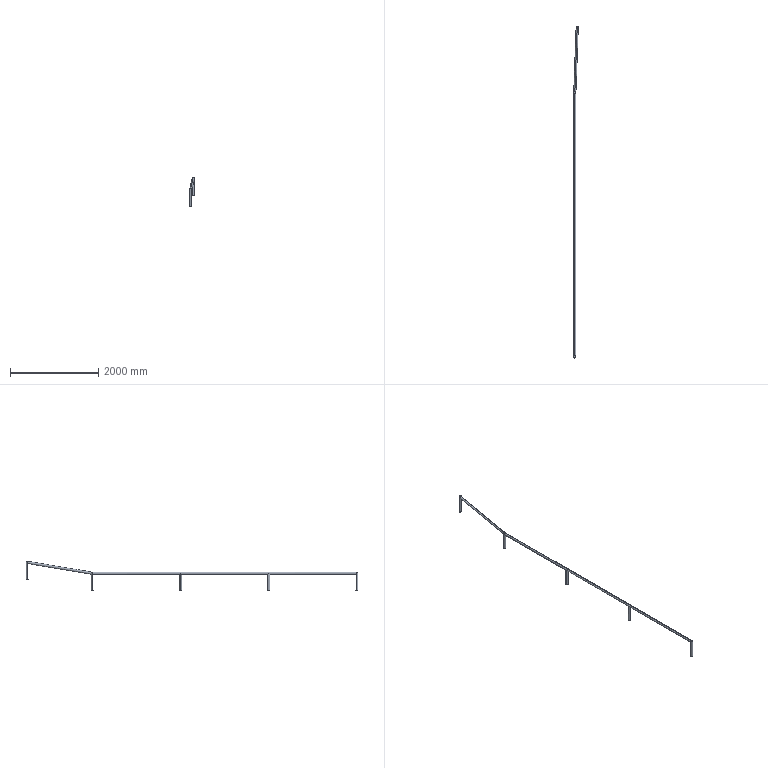Part | STEP file | Guide 2_default<machined> | 7 solids | 29 faces | box 103.693 x 7528 x 678.002 mm | volume 18500924 mm3 | cylinder 21 | plane 8 | commonest cylinder face diameters 50 x21